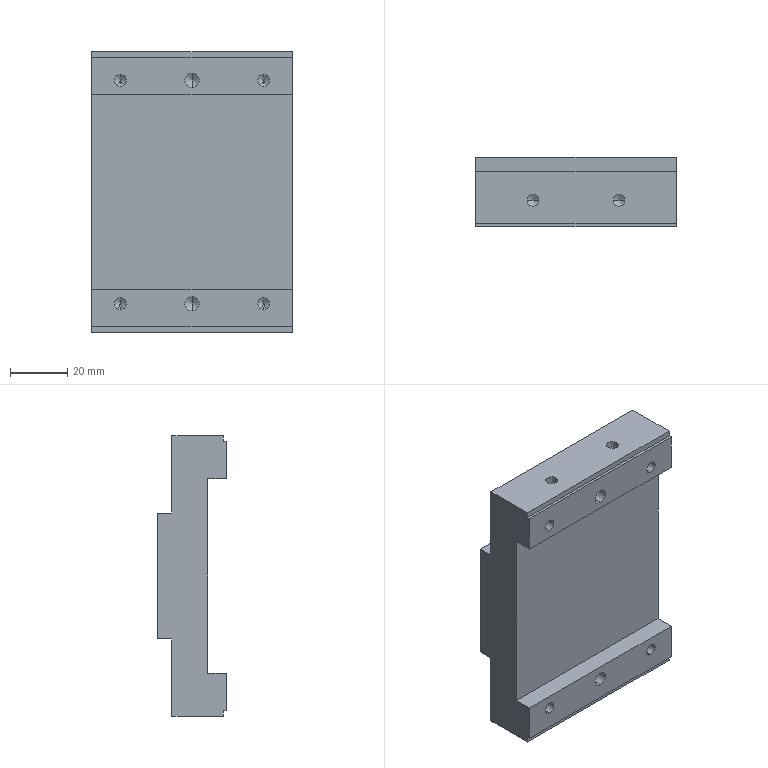Part | SolidWorks | features BaseBody 1 | 1 solid | 65 faces | box 70 x 24 x 98 mm | volume 112077 mm3 | cylinder 24 | cone 22 | plane 19 | commonest cylinder face diameters 4.134 x16 5 x4 3 x2 5.5 x2